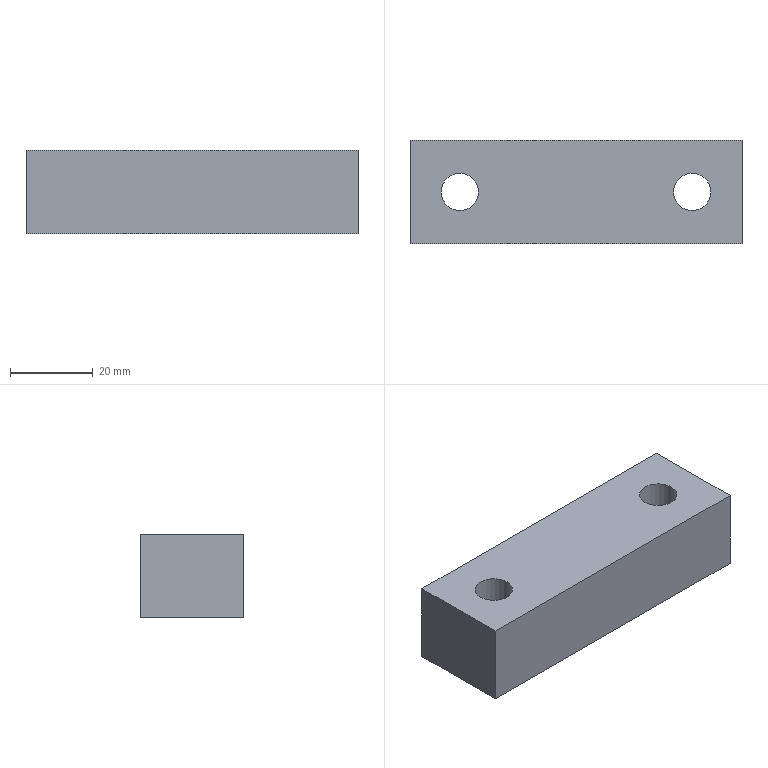Part | STEP file | lll_id562_x_t | 1 solid | 12 faces | box 80 x 25 x 20 mm | volume 35216 mm3 | plane 8 | cylinder 4 | commonest cylinder face diameters 9.009 x2 14.507 x2
STEP:
#1=CARTESIAN_POINT('',(222.689,389.5,0.));
#2=VERTEX_POINT('',#1);
#3=CARTESIAN_POINT('',(215.435,389.5,0.));
#4=DIRECTION('',(0.,0.,1.));
#5=DIRECTION('',(1.,0.,0.));
#6=AXIS2_PLACEMENT_3D('',#3,#4,#5);
#7=CIRCLE('',#6,7.253);
#8=EDGE_CURVE('',#2,#2,#7,.T.);
#9=ORIENTED_EDGE('',*,*,#8,.T.);
#10=EDGE_LOOP('',(#9));
#11=FACE_BOUND('',#10,.T.);
#12=CARTESIAN_POINT('',(283.435,377.,0.));
#13=VERTEX_POINT('',#12);
#14=CARTESIAN_POINT('',(283.435,402.,0.));
#15=VERTEX_POINT('',#14);
#16=CARTESIAN_POINT('',(283.435,389.5,0.));
#17=DIRECTION('',(0.,1.,0.));
#18=VECTOR('',#17,1.);
#19=LINE('',#16,#18);
#20=EDGE_CURVE('',#13,#15,#19,.T.);
#21=ORIENTED_EDGE('',*,*,#20,.F.);
#22=CARTESIAN_POINT('',(203.435,377.,0.));
#23=VERTEX_POINT('',#22);
#24=CARTESIAN_POINT('',(270.935,377.,0.));
#25=DIRECTION('',(1.,0.,0.));
#26=VECTOR('',#25,1.);
#27=LINE('',#24,#26);
#28=EDGE_CURVE('',#23,#13,#27,.T.);
#29=ORIENTED_EDGE('',*,*,#28,.F.);
#30=CARTESIAN_POINT('',(203.435,402.,0.));
#31=VERTEX_POINT('',#30);
#32=CARTESIAN_POINT('',(203.435,389.5,0.));
#33=DIRECTION('',(0.,-1.,0.));
#34=VECTOR('',#33,1.);
#35=LINE('',#32,#34);
#36=EDGE_CURVE('',#31,#23,#35,.T.);
#37=ORIENTED_EDGE('',*,*,#36,.F.);
#38=CARTESIAN_POINT('',(270.935,402.,0.));
#39=DIRECTION('',(-1.,0.,0.));
#40=VECTOR('',#39,1.);
#41=LINE('',#38,#40);
#42=EDGE_CURVE('',#15,#31,#41,.T.);
#43=ORIENTED_EDGE('',*,*,#42,.F.);
#44=EDGE_LOOP('',(#21,#29,#37,#43));
#45=FACE_BOUND('',#44,.T.);
#46=CARTESIAN_POINT('',(278.689,389.5,0.));
#47=VERTEX_POINT('',#46);
#48=CARTESIAN_POINT('',(271.435,389.5,0.));
#49=DIRECTION('',(0.,0.,1.));
#50=DIRECTION('',(1.,0.,0.));
#51=AXIS2_PLACEMENT_3D('',#48,#49,#50);
#52=CIRCLE('',#51,7.253);
#53=EDGE_CURVE('',#47,#47,#52,.T.);
#54=ORIENTED_EDGE('',*,*,#53,.T.);
#55=EDGE_LOOP('',(#54));
#56=FACE_BOUND('',#55,.T.);
#57=CARTESIAN_POINT('',(270.935,389.5,0.));
#58=DIRECTION('',(0.,0.,-1.));
#59=DIRECTION('',(-1.,0.,0.));
#60=AXIS2_PLACEMENT_3D('',#57,#58,#59);
#61=PLANE('',#60);
#62=ADVANCED_FACE('',(#11,#45,#56),#61,.T.);
#63=CARTESIAN_POINT('',(275.94,389.5,20.));
#64=VERTEX_POINT('',#63);
#65=CARTESIAN_POINT('',(271.435,389.5,20.));
#66=DIRECTION('',(0.,0.,1.));
#67=DIRECTION('',(1.,0.,0.));
#68=AXIS2_PLACEMENT_3D('',#65,#66,#67);
#69=CIRCLE('',#68,4.505);
#70=EDGE_CURVE('',#64,#64,#69,.T.);
#71=ORIENTED_EDGE('',*,*,#70,.F.);
#72=EDGE_LOOP('',(#71));
#73=FACE_BOUND('',#72,.T.);
#74=CARTESIAN_POINT('',(219.94,389.5,20.));
#75=VERTEX_POINT('',#74);
#76=CARTESIAN_POINT('',(215.435,389.5,20.));
#77=DIRECTION('',(0.,0.,1.));
#78=DIRECTION('',(1.,0.,0.));
#79=AXIS2_PLACEMENT_3D('',#76,#77,#78);
#80=CIRCLE('',#79,4.505);
#81=EDGE_CURVE('',#75,#75,#80,.T.);
#82=ORIENTED_EDGE('',*,*,#81,.F.);
#83=EDGE_LOOP('',(#82));
#84=FACE_BOUND('',#83,.T.);
#85=CARTESIAN_POINT('',(283.435,377.,20.));
#86=VERTEX_POINT('',#85);
#87=CARTESIAN_POINT('',(203.435,377.,20.));
#88=VERTEX_POINT('',#87);
#89=CARTESIAN_POINT('',(270.935,377.,20.));
#90=DIRECTION('',(-1.,0.,0.));
#91=VECTOR('',#90,1.);
#92=LINE('',#89,#91);
#93=EDGE_CURVE('',#86,#88,#92,.T.);
#94=ORIENTED_EDGE('',*,*,#93,.F.);
#95=CARTESIAN_POINT('',(283.435,402.,20.));
#96=VERTEX_POINT('',#95);
#97=CARTESIAN_POINT('',(283.435,389.5,20.));
#98=DIRECTION('',(0.,-1.,0.));
#99=VECTOR('',#98,1.);
#100=LINE('',#97,#99);
#101=EDGE_CURVE('',#96,#86,#100,.T.);
#102=ORIENTED_EDGE('',*,*,#101,.F.);
#103=CARTESIAN_POINT('',(203.435,402.,20.));
#104=VERTEX_POINT('',#103);
#105=CARTESIAN_POINT('',(270.935,402.,20.));
#106=DIRECTION('',(1.,0.,0.));
#107=VECTOR('',#106,1.);
#108=LINE('',#105,#107);
#109=EDGE_CURVE('',#104,#96,#108,.T.);
#110=ORIENTED_EDGE('',*,*,#109,.F.);
#111=CARTESIAN_POINT('',(203.435,389.5,20.));
#112=DIRECTION('',(0.,1.,0.));
#113=VECTOR('',#112,1.);
#114=LINE('',#111,#113);
#115=EDGE_CURVE('',#88,#104,#114,.T.);
#116=ORIENTED_EDGE('',*,*,#115,.F.);
#117=EDGE_LOOP('',(#94,#102,#110,#116));
#118=FACE_BOUND('',#117,.T.);
#119=CARTESIAN_POINT('',(270.935,389.5,20.));
#120=DIRECTION('',(0.,0.,1.));
#121=DIRECTION('',(1.,0.,0.));
#122=AXIS2_PLACEMENT_3D('',#119,#120,#121);
#123=PLANE('',#122);
#124=ADVANCED_FACE('',(#73,#84,#118),#123,.T.);
#125=CARTESIAN_POINT('',(283.435,377.,0.));
#126=DIRECTION('',(0.,0.,1.));
#127=VECTOR('',#126,1.);
#128=LINE('',#125,#127);
#129=EDGE_CURVE('',#13,#86,#128,.T.);
#130=ORIENTED_EDGE('',*,*,#129,.T.);
#131=ORIENTED_EDGE('',*,*,#93,.T.);
#132=CARTESIAN_POINT('',(203.435,377.,0.));
#133=DIRECTION('',(0.,0.,1.));
#134=VECTOR('',#133,1.);
#135=LINE('',#132,#134);
#136=EDGE_CURVE('',#23,#88,#135,.T.);
#137=ORIENTED_EDGE('',*,*,#136,.F.);
#138=ORIENTED_EDGE('',*,*,#28,.T.);
#139=EDGE_LOOP('',(#130,#131,#137,#138));
#140=FACE_OUTER_BOUND('',#139,.T.);
#141=CARTESIAN_POINT('',(270.935,377.,0.));
#142=DIRECTION('',(0.,-1.,0.));
#143=DIRECTION('',(0.,0.,-1.));
#144=AXIS2_PLACEMENT_3D('',#141,#142,#143);
#145=PLANE('',#144);
#146=ADVANCED_FACE('',(#140),#145,.T.);
#147=ORIENTED_EDGE('',*,*,#42,.T.);
#148=CARTESIAN_POINT('',(203.435,402.,0.));
#149=DIRECTION('',(0.,0.,1.));
#150=VECTOR('',#149,1.);
#151=LINE('',#148,#150);
#152=EDGE_CURVE('',#31,#104,#151,.T.);
#153=ORIENTED_EDGE('',*,*,#152,.T.);
#154=ORIENTED_EDGE('',*,*,#109,.T.);
#155=CARTESIAN_POINT('',(283.435,402.,0.));
#156=DIRECTION('',(0.,0.,1.));
#157=VECTOR('',#156,1.);
#158=LINE('',#155,#157);
#159=EDGE_CURVE('',#15,#96,#158,.T.);
#160=ORIENTED_EDGE('',*,*,#159,.F.);
#161=EDGE_LOOP('',(#147,#153,#154,#160));
#162=FACE_OUTER_BOUND('',#161,.T.);
#163=CARTESIAN_POINT('',(270.935,402.,0.));
#164=DIRECTION('',(0.,1.,0.));
#165=DIRECTION('',(0.,0.,1.));
#166=AXIS2_PLACEMENT_3D('',#163,#164,#165);
#167=PLANE('',#166);
#168=ADVANCED_FACE('',(#162),#167,.T.);
#169=ORIENTED_EDGE('',*,*,#20,.T.);
#170=ORIENTED_EDGE('',*,*,#159,.T.);
#171=ORIENTED_EDGE('',*,*,#101,.T.);
#172=ORIENTED_EDGE('',*,*,#129,.F.);
#173=EDGE_LOOP('',(#169,#170,#171,#172));
#174=FACE_OUTER_BOUND('',#173,.T.);
#175=CARTESIAN_POINT('',(283.435,389.5,0.));
#176=DIRECTION('',(1.,0.,0.));
#177=DIRECTION('',(0.,0.,-1.));
#178=AXIS2_PLACEMENT_3D('',#175,#176,#177);
#179=PLANE('',#178);
#180=ADVANCED_FACE('',(#174),#179,.T.);
#181=ORIENTED_EDGE('',*,*,#136,.T.);
#182=ORIENTED_EDGE('',*,*,#115,.T.);
#183=ORIENTED_EDGE('',*,*,#152,.F.);
#184=ORIENTED_EDGE('',*,*,#36,.T.);
#185=EDGE_LOOP('',(#181,#182,#183,#184));
#186=FACE_OUTER_BOUND('',#185,.T.);
#187=CARTESIAN_POINT('',(203.435,389.5,0.));
#188=DIRECTION('',(-1.,0.,0.));
#189=DIRECTION('',(0.,0.,1.));
#190=AXIS2_PLACEMENT_3D('',#187,#188,#189);
#191=PLANE('',#190);
#192=ADVANCED_FACE('',(#186),#191,.T.);
#193=ORIENTED_EDGE('',*,*,#81,.T.);
#194=EDGE_LOOP('',(#193));
#195=FACE_BOUND('',#194,.T.);
#196=CARTESIAN_POINT('',(219.94,389.5,11.));
#197=VERTEX_POINT('',#196);
#198=CARTESIAN_POINT('',(215.435,389.5,11.));
#199=DIRECTION('',(0.,0.,1.));
#200=DIRECTION('',(1.,0.,0.));
#201=AXIS2_PLACEMENT_3D('',#198,#199,#200);
#202=CIRCLE('',#201,4.505);
#203=EDGE_CURVE('',#197,#197,#202,.T.);
#204=ORIENTED_EDGE('',*,*,#203,.F.);
#205=EDGE_LOOP('',(#204));
#206=FACE_BOUND('',#205,.T.);
#207=CARTESIAN_POINT('',(215.435,389.5,-5.));
#208=DIRECTION('',(0.,0.,1.));
#209=DIRECTION('',(-1.,0.,0.));
#210=AXIS2_PLACEMENT_3D('',#207,#208,#209);
#211=CYLINDRICAL_SURFACE('',#210,4.505);
#212=ADVANCED_FACE('',(#195,#206),#211,.F.);
#213=ORIENTED_EDGE('',*,*,#203,.T.);
#214=EDGE_LOOP('',(#213));
#215=FACE_BOUND('',#214,.T.);
#216=CARTESIAN_POINT('',(222.689,389.5,11.));
#217=VERTEX_POINT('',#216);
#218=CARTESIAN_POINT('',(215.435,389.5,11.));
#219=DIRECTION('',(0.,0.,1.));
#220=DIRECTION('',(1.,0.,0.));
#221=AXIS2_PLACEMENT_3D('',#218,#219,#220);
#222=CIRCLE('',#221,7.253);
#223=EDGE_CURVE('',#217,#217,#222,.T.);
#224=ORIENTED_EDGE('',*,*,#223,.F.);
#225=EDGE_LOOP('',(#224));
#226=FACE_BOUND('',#225,.T.);
#227=CARTESIAN_POINT('',(215.435,389.5,11.));
#228=DIRECTION('',(0.,0.,1.));
#229=DIRECTION('',(-1.,0.,0.));
#230=AXIS2_PLACEMENT_3D('',#227,#228,#229);
#231=PLANE('',#230);
#232=ADVANCED_FACE('',(#215,#226),#231,.F.);
#233=ORIENTED_EDGE('',*,*,#223,.T.);
#234=EDGE_LOOP('',(#233));
#235=FACE_BOUND('',#234,.T.);
#236=ORIENTED_EDGE('',*,*,#8,.F.);
#237=EDGE_LOOP('',(#236));
#238=FACE_BOUND('',#237,.T.);
#239=CARTESIAN_POINT('',(215.435,389.5,0.));
#240=DIRECTION('',(0.,0.,1.));
#241=DIRECTION('',(-1.,0.,0.));
#242=AXIS2_PLACEMENT_3D('',#239,#240,#241);
#243=CYLINDRICAL_SURFACE('',#242,7.253);
#244=ADVANCED_FACE('',(#235,#238),#243,.F.);
#245=ORIENTED_EDGE('',*,*,#70,.T.);
#246=EDGE_LOOP('',(#245));
#247=FACE_BOUND('',#246,.T.);
#248=CARTESIAN_POINT('',(275.94,389.5,11.));
#249=VERTEX_POINT('',#248);
#250=CARTESIAN_POINT('',(271.435,389.5,11.));
#251=DIRECTION('',(0.,0.,1.));
#252=DIRECTION('',(1.,0.,0.));
#253=AXIS2_PLACEMENT_3D('',#250,#251,#252);
#254=CIRCLE('',#253,4.505);
#255=EDGE_CURVE('',#249,#249,#254,.T.);
#256=ORIENTED_EDGE('',*,*,#255,.F.);
#257=EDGE_LOOP('',(#256));
#258=FACE_BOUND('',#257,.T.);
#259=CARTESIAN_POINT('',(271.435,389.5,-5.));
#260=DIRECTION('',(0.,0.,1.));
#261=DIRECTION('',(-1.,0.,0.));
#262=AXIS2_PLACEMENT_3D('',#259,#260,#261);
#263=CYLINDRICAL_SURFACE('',#262,4.505);
#264=ADVANCED_FACE('',(#247,#258),#263,.F.);
#265=ORIENTED_EDGE('',*,*,#255,.T.);
#266=EDGE_LOOP('',(#265));
#267=FACE_BOUND('',#266,.T.);
#268=CARTESIAN_POINT('',(278.689,389.5,11.));
#269=VERTEX_POINT('',#268);
#270=CARTESIAN_POINT('',(271.435,389.5,11.));
#271=DIRECTION('',(0.,0.,1.));
#272=DIRECTION('',(1.,0.,0.));
#273=AXIS2_PLACEMENT_3D('',#270,#271,#272);
#274=CIRCLE('',#273,7.253);
#275=EDGE_CURVE('',#269,#269,#274,.T.);
#276=ORIENTED_EDGE('',*,*,#275,.F.);
#277=EDGE_LOOP('',(#276));
#278=FACE_BOUND('',#277,.T.);
#279=CARTESIAN_POINT('',(271.435,389.5,11.));
#280=DIRECTION('',(0.,0.,1.));
#281=DIRECTION('',(-1.,0.,0.));
#282=AXIS2_PLACEMENT_3D('',#279,#280,#281);
#283=PLANE('',#282);
#284=ADVANCED_FACE('',(#267,#278),#283,.F.);
#285=ORIENTED_EDGE('',*,*,#275,.T.);
#286=EDGE_LOOP('',(#285));
#287=FACE_BOUND('',#286,.T.);
#288=ORIENTED_EDGE('',*,*,#53,.F.);
#289=EDGE_LOOP('',(#288));
#290=FACE_BOUND('',#289,.T.);
#291=CARTESIAN_POINT('',(271.435,389.5,0.));
#292=DIRECTION('',(0.,0.,1.));
#293=DIRECTION('',(-1.,0.,0.));
#294=AXIS2_PLACEMENT_3D('',#291,#292,#293);
#295=CYLINDRICAL_SURFACE('',#294,7.253);
#296=ADVANCED_FACE('',(#287,#290),#295,.F.);
#297=CLOSED_SHELL('',(#62,#124,#146,#168,#180,#192,#212,#232,#244,#264,#284,#296));
#298=MANIFOLD_SOLID_BREP('',#297);
#299=(LENGTH_UNIT()NAMED_UNIT(*)SI_UNIT(.MILLI.,.METRE.));
#300=UNCERTAINTY_MEASURE_WITH_UNIT(LENGTH_MEASURE(0.00002),#299,'','');
#301=(NAMED_UNIT(*)PLANE_ANGLE_UNIT()SI_UNIT($,.RADIAN.));
#302=PLANE_ANGLE_MEASURE_WITH_UNIT(PLANE_ANGLE_MEASURE(0.01745),#301);
#303=DIMENSIONAL_EXPONENTS(0.,0.,0.,0.,0.,0.,0.);
#304=(CONVERSION_BASED_UNIT('DEGREE',#302)NAMED_UNIT(#303)PLANE_ANGLE_UNIT());
#305=(NAMED_UNIT(*)SI_UNIT($,.STERADIAN.)SOLID_ANGLE_UNIT());
#306=(GEOMETRIC_REPRESENTATION_CONTEXT(3)GLOBAL_UNCERTAINTY_ASSIGNED_CONTEXT((#300))GLOBAL_UNIT_ASSIGNED_CONTEXT((#299,#304,#305))REPRESENTATION_CONTEXT('',''));
#307=ADVANCED_BREP_SHAPE_REPRESENTATION('',(#298),#306);